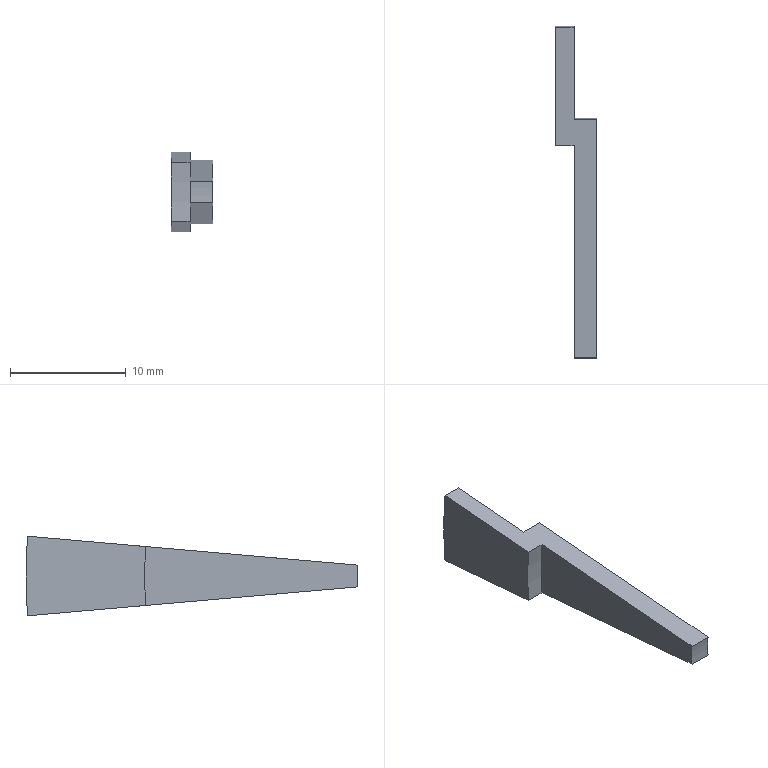Part | SolidWorks | features Revolution 1 | 1 solid | 10 faces | box 3.582 x 28.652 x 6.869 mm | volume 248.306 mm3 | plane 6 | cylinder 4 | commonest cylinder face diameters 21.59 x1 58.326 x1 62.852 x1 78.811 x1
STEP:
#1=CARTESIAN_POINT('',(-109.954,39.256,-3.434));
#2=VERTEX_POINT('',#1);
#3=CARTESIAN_POINT('',(-109.954,39.256,3.434));
#4=VERTEX_POINT('',#3);
#5=CARTESIAN_POINT('',(-109.954,0.,0.));
#6=DIRECTION('',(1.,0.,0.));
#7=DIRECTION('',(0.,0.,-1.));
#8=AXIS2_PLACEMENT_3D('',#5,#6,#7);
#9=CIRCLE('',#8,39.406);
#10=EDGE_CURVE('',#2,#4,#9,.T.);
#11=ORIENTED_EDGE('',*,*,#10,.F.);
#12=CARTESIAN_POINT('',(-111.582,39.256,-3.434));
#13=VERTEX_POINT('',#12);
#14=CARTESIAN_POINT('',(-111.582,39.256,-3.434));
#15=DIRECTION('',(-1.,0.,0.));
#16=VECTOR('',#15,1000.);
#17=LINE('',#14,#16);
#18=EDGE_CURVE('',#2,#13,#17,.T.);
#19=ORIENTED_EDGE('',*,*,#18,.T.);
#20=CARTESIAN_POINT('',(-111.582,39.256,3.434));
#21=VERTEX_POINT('',#20);
#22=CARTESIAN_POINT('',(-111.582,0.,0.));
#23=DIRECTION('',(1.,0.,0.));
#24=DIRECTION('',(0.,0.,-1.));
#25=AXIS2_PLACEMENT_3D('',#22,#23,#24);
#26=CIRCLE('',#25,39.406);
#27=EDGE_CURVE('',#13,#21,#26,.T.);
#28=ORIENTED_EDGE('',*,*,#27,.T.);
#29=CARTESIAN_POINT('',(-111.582,39.256,3.434));
#30=DIRECTION('',(-1.,0.,0.));
#31=VECTOR('',#30,1000.);
#32=LINE('',#29,#31);
#33=EDGE_CURVE('',#4,#21,#32,.T.);
#34=ORIENTED_EDGE('',*,*,#33,.F.);
#35=EDGE_LOOP('',(#11,#19,#28,#34));
#36=FACE_OUTER_BOUND('',#35,.T.);
#37=CARTESIAN_POINT('',(0.,0.,0.));
#38=DIRECTION('',(1.,0.,0.));
#39=DIRECTION('',(0.,0.,-1.));
#40=AXIS2_PLACEMENT_3D('',#37,#38,#39);
#41=CYLINDRICAL_SURFACE('',#40,39.406);
#42=ADVANCED_FACE('',(#36),#41,.T.);
#43=CARTESIAN_POINT('',(-109.954,31.306,-2.739));
#44=VERTEX_POINT('',#43);
#45=CARTESIAN_POINT('',(-109.954,31.306,2.739));
#46=VERTEX_POINT('',#45);
#47=CARTESIAN_POINT('',(-109.954,0.,0.));
#48=DIRECTION('',(1.,0.,0.));
#49=DIRECTION('',(0.,0.,-1.));
#50=AXIS2_PLACEMENT_3D('',#47,#48,#49);
#51=CIRCLE('',#50,31.426);
#52=EDGE_CURVE('',#44,#46,#51,.T.);
#53=ORIENTED_EDGE('',*,*,#52,.F.);
#54=CARTESIAN_POINT('',(-109.954,39.256,-3.434));
#55=DIRECTION('',(0.,0.9962,-0.08716));
#56=VECTOR('',#55,1000.);
#57=LINE('',#54,#56);
#58=EDGE_CURVE('',#44,#2,#57,.T.);
#59=ORIENTED_EDGE('',*,*,#58,.T.);
#60=ORIENTED_EDGE('',*,*,#10,.T.);
#61=CARTESIAN_POINT('',(-109.954,39.256,3.434));
#62=DIRECTION('',(0.,0.9962,0.08716));
#63=VECTOR('',#62,1000.);
#64=LINE('',#61,#63);
#65=EDGE_CURVE('',#46,#4,#64,.T.);
#66=ORIENTED_EDGE('',*,*,#65,.F.);
#67=EDGE_LOOP('',(#53,#59,#60,#66));
#68=FACE_OUTER_BOUND('',#67,.T.);
#69=CARTESIAN_POINT('',(-109.954,39.256,-3.434));
#70=DIRECTION('',(1.,0.,0.));
#71=DIRECTION('',(0.,0.,-1.));
#72=AXIS2_PLACEMENT_3D('',#69,#70,#71);
#73=PLANE('',#72);
#74=ADVANCED_FACE('',(#68),#73,.T.);
#75=CARTESIAN_POINT('',(-108.,31.306,-2.739));
#76=VERTEX_POINT('',#75);
#77=CARTESIAN_POINT('',(-108.,31.306,2.739));
#78=VERTEX_POINT('',#77);
#79=CARTESIAN_POINT('',(-108.,0.,0.));
#80=DIRECTION('',(1.,0.,0.));
#81=DIRECTION('',(0.,0.,-1.));
#82=AXIS2_PLACEMENT_3D('',#79,#80,#81);
#83=CIRCLE('',#82,31.426);
#84=EDGE_CURVE('',#76,#78,#83,.T.);
#85=ORIENTED_EDGE('',*,*,#84,.F.);
#86=CARTESIAN_POINT('',(-109.954,31.306,-2.739));
#87=DIRECTION('',(-1.,0.,0.));
#88=VECTOR('',#87,1000.);
#89=LINE('',#86,#88);
#90=EDGE_CURVE('',#76,#44,#89,.T.);
#91=ORIENTED_EDGE('',*,*,#90,.T.);
#92=ORIENTED_EDGE('',*,*,#52,.T.);
#93=CARTESIAN_POINT('',(-109.954,31.306,2.739));
#94=DIRECTION('',(-1.,0.,0.));
#95=VECTOR('',#94,1000.);
#96=LINE('',#93,#95);
#97=EDGE_CURVE('',#78,#46,#96,.T.);
#98=ORIENTED_EDGE('',*,*,#97,.F.);
#99=EDGE_LOOP('',(#85,#91,#92,#98));
#100=FACE_OUTER_BOUND('',#99,.T.);
#101=CARTESIAN_POINT('',(0.,0.,0.));
#102=DIRECTION('',(1.,0.,0.));
#103=DIRECTION('',(0.,0.,-1.));
#104=AXIS2_PLACEMENT_3D('',#101,#102,#103);
#105=CYLINDRICAL_SURFACE('',#104,31.426);
#106=ADVANCED_FACE('',(#100),#105,.T.);
#107=CARTESIAN_POINT('',(-108.,10.754,-0.9408));
#108=VERTEX_POINT('',#107);
#109=CARTESIAN_POINT('',(-108.,10.754,0.9408));
#110=VERTEX_POINT('',#109);
#111=CARTESIAN_POINT('',(-108.,0.,0.));
#112=DIRECTION('',(1.,0.,0.));
#113=DIRECTION('',(0.,0.,-1.));
#114=AXIS2_PLACEMENT_3D('',#111,#112,#113);
#115=CIRCLE('',#114,10.795);
#116=EDGE_CURVE('',#108,#110,#115,.T.);
#117=ORIENTED_EDGE('',*,*,#116,.F.);
#118=CARTESIAN_POINT('',(-108.,31.306,-2.739));
#119=DIRECTION('',(0.,0.9962,-0.08716));
#120=VECTOR('',#119,1000.);
#121=LINE('',#118,#120);
#122=EDGE_CURVE('',#108,#76,#121,.T.);
#123=ORIENTED_EDGE('',*,*,#122,.T.);
#124=ORIENTED_EDGE('',*,*,#84,.T.);
#125=CARTESIAN_POINT('',(-108.,31.306,2.739));
#126=DIRECTION('',(0.,0.9962,0.08716));
#127=VECTOR('',#126,1000.);
#128=LINE('',#125,#127);
#129=EDGE_CURVE('',#110,#78,#128,.T.);
#130=ORIENTED_EDGE('',*,*,#129,.F.);
#131=EDGE_LOOP('',(#117,#123,#124,#130));
#132=FACE_OUTER_BOUND('',#131,.T.);
#133=CARTESIAN_POINT('',(-108.,31.306,-2.739));
#134=DIRECTION('',(1.,0.,0.));
#135=DIRECTION('',(0.,0.,-1.));
#136=AXIS2_PLACEMENT_3D('',#133,#134,#135);
#137=PLANE('',#136);
#138=ADVANCED_FACE('',(#132),#137,.T.);
#139=CARTESIAN_POINT('',(-109.954,10.754,-0.9408));
#140=VERTEX_POINT('',#139);
#141=CARTESIAN_POINT('',(-109.954,10.754,0.9408));
#142=VERTEX_POINT('',#141);
#143=CARTESIAN_POINT('',(-109.954,0.,0.));
#144=DIRECTION('',(1.,0.,0.));
#145=DIRECTION('',(0.,0.,-1.));
#146=AXIS2_PLACEMENT_3D('',#143,#144,#145);
#147=CIRCLE('',#146,10.795);
#148=EDGE_CURVE('',#140,#142,#147,.T.);
#149=ORIENTED_EDGE('',*,*,#148,.F.);
#150=CARTESIAN_POINT('',(-108.,10.754,-0.9408));
#151=DIRECTION('',(1.,0.,0.));
#152=VECTOR('',#151,1000.);
#153=LINE('',#150,#152);
#154=EDGE_CURVE('',#140,#108,#153,.T.);
#155=ORIENTED_EDGE('',*,*,#154,.T.);
#156=ORIENTED_EDGE('',*,*,#116,.T.);
#157=CARTESIAN_POINT('',(-108.,10.754,0.9408));
#158=DIRECTION('',(1.,0.,0.));
#159=VECTOR('',#158,1000.);
#160=LINE('',#157,#159);
#161=EDGE_CURVE('',#142,#110,#160,.T.);
#162=ORIENTED_EDGE('',*,*,#161,.F.);
#163=EDGE_LOOP('',(#149,#155,#156,#162));
#164=FACE_OUTER_BOUND('',#163,.T.);
#165=CARTESIAN_POINT('',(0.,0.,0.));
#166=DIRECTION('',(1.,0.,0.));
#167=DIRECTION('',(0.,0.,-1.));
#168=AXIS2_PLACEMENT_3D('',#165,#166,#167);
#169=CYLINDRICAL_SURFACE('',#168,10.795);
#170=ADVANCED_FACE('',(#164),#169,.F.);
#171=CARTESIAN_POINT('',(-109.954,29.052,-2.542));
#172=VERTEX_POINT('',#171);
#173=CARTESIAN_POINT('',(-109.954,29.052,2.542));
#174=VERTEX_POINT('',#173);
#175=CARTESIAN_POINT('',(-109.954,0.,0.));
#176=DIRECTION('',(1.,0.,0.));
#177=DIRECTION('',(0.,0.,-1.));
#178=AXIS2_PLACEMENT_3D('',#175,#176,#177);
#179=CIRCLE('',#178,29.163);
#180=EDGE_CURVE('',#172,#174,#179,.T.);
#181=ORIENTED_EDGE('',*,*,#180,.F.);
#182=CARTESIAN_POINT('',(-109.954,29.052,-2.542));
#183=DIRECTION('',(0.,-0.9962,0.08716));
#184=VECTOR('',#183,1000.);
#185=LINE('',#182,#184);
#186=EDGE_CURVE('',#172,#140,#185,.T.);
#187=ORIENTED_EDGE('',*,*,#186,.T.);
#188=ORIENTED_EDGE('',*,*,#148,.T.);
#189=CARTESIAN_POINT('',(-109.954,29.052,2.542));
#190=DIRECTION('',(0.,-0.9962,-0.08716));
#191=VECTOR('',#190,1000.);
#192=LINE('',#189,#191);
#193=EDGE_CURVE('',#174,#142,#192,.T.);
#194=ORIENTED_EDGE('',*,*,#193,.F.);
#195=EDGE_LOOP('',(#181,#187,#188,#194));
#196=FACE_OUTER_BOUND('',#195,.T.);
#197=CARTESIAN_POINT('',(-109.954,29.052,-2.542));
#198=DIRECTION('',(-1.,0.,0.));
#199=DIRECTION('',(0.,0.,1.));
#200=AXIS2_PLACEMENT_3D('',#197,#198,#199);
#201=PLANE('',#200);
#202=ADVANCED_FACE('',(#196),#201,.T.);
#203=CARTESIAN_POINT('',(-111.582,29.052,-2.542));
#204=VERTEX_POINT('',#203);
#205=CARTESIAN_POINT('',(-111.582,29.052,2.542));
#206=VERTEX_POINT('',#205);
#207=CARTESIAN_POINT('',(-111.582,0.,0.));
#208=DIRECTION('',(1.,0.,0.));
#209=DIRECTION('',(0.,0.,-1.));
#210=AXIS2_PLACEMENT_3D('',#207,#208,#209);
#211=CIRCLE('',#210,29.163);
#212=EDGE_CURVE('',#204,#206,#211,.T.);
#213=ORIENTED_EDGE('',*,*,#212,.F.);
#214=CARTESIAN_POINT('',(-111.582,29.052,-2.542));
#215=DIRECTION('',(1.,0.,0.));
#216=VECTOR('',#215,1000.);
#217=LINE('',#214,#216);
#218=EDGE_CURVE('',#204,#172,#217,.T.);
#219=ORIENTED_EDGE('',*,*,#218,.T.);
#220=ORIENTED_EDGE('',*,*,#180,.T.);
#221=CARTESIAN_POINT('',(-111.582,29.052,2.542));
#222=DIRECTION('',(1.,0.,0.));
#223=VECTOR('',#222,1000.);
#224=LINE('',#221,#223);
#225=EDGE_CURVE('',#206,#174,#224,.T.);
#226=ORIENTED_EDGE('',*,*,#225,.F.);
#227=EDGE_LOOP('',(#213,#219,#220,#226));
#228=FACE_OUTER_BOUND('',#227,.T.);
#229=CARTESIAN_POINT('',(0.,0.,0.));
#230=DIRECTION('',(1.,0.,0.));
#231=DIRECTION('',(0.,0.,-1.));
#232=AXIS2_PLACEMENT_3D('',#229,#230,#231);
#233=CYLINDRICAL_SURFACE('',#232,29.163);
#234=ADVANCED_FACE('',(#228),#233,.F.);
#235=CARTESIAN_POINT('',(-111.582,29.052,-2.542));
#236=DIRECTION('',(0.,-0.9962,0.08716));
#237=VECTOR('',#236,1000.);
#238=LINE('',#235,#237);
#239=EDGE_CURVE('',#13,#204,#238,.T.);
#240=ORIENTED_EDGE('',*,*,#239,.T.);
#241=ORIENTED_EDGE('',*,*,#212,.T.);
#242=CARTESIAN_POINT('',(-111.582,29.052,2.542));
#243=DIRECTION('',(0.,-0.9962,-0.08716));
#244=VECTOR('',#243,1000.);
#245=LINE('',#242,#244);
#246=EDGE_CURVE('',#21,#206,#245,.T.);
#247=ORIENTED_EDGE('',*,*,#246,.F.);
#248=ORIENTED_EDGE('',*,*,#27,.F.);
#249=EDGE_LOOP('',(#240,#241,#247,#248));
#250=FACE_OUTER_BOUND('',#249,.T.);
#251=CARTESIAN_POINT('',(-111.582,29.052,-2.542));
#252=DIRECTION('',(-1.,0.,0.));
#253=DIRECTION('',(0.,0.,1.));
#254=AXIS2_PLACEMENT_3D('',#251,#252,#253);
#255=PLANE('',#254);
#256=ADVANCED_FACE('',(#250),#255,.T.);
#257=ORIENTED_EDGE('',*,*,#18,.F.);
#258=ORIENTED_EDGE('',*,*,#58,.F.);
#259=ORIENTED_EDGE('',*,*,#90,.F.);
#260=ORIENTED_EDGE('',*,*,#122,.F.);
#261=ORIENTED_EDGE('',*,*,#154,.F.);
#262=ORIENTED_EDGE('',*,*,#186,.F.);
#263=ORIENTED_EDGE('',*,*,#218,.F.);
#264=ORIENTED_EDGE('',*,*,#239,.F.);
#265=EDGE_LOOP('',(#257,#258,#259,#260,#261,#262,#263,#264));
#266=FACE_OUTER_BOUND('',#265,.T.);
#267=CARTESIAN_POINT('',(0.,0.,0.));
#268=DIRECTION('',(0.,-0.08716,-0.9962));
#269=DIRECTION('',(-1.,0.,0.));
#270=AXIS2_PLACEMENT_3D('',#267,#268,#269);
#271=PLANE('',#270);
#272=ADVANCED_FACE('',(#266),#271,.T.);
#273=ORIENTED_EDGE('',*,*,#33,.T.);
#274=ORIENTED_EDGE('',*,*,#246,.T.);
#275=ORIENTED_EDGE('',*,*,#225,.T.);
#276=ORIENTED_EDGE('',*,*,#193,.T.);
#277=ORIENTED_EDGE('',*,*,#161,.T.);
#278=ORIENTED_EDGE('',*,*,#129,.T.);
#279=ORIENTED_EDGE('',*,*,#97,.T.);
#280=ORIENTED_EDGE('',*,*,#65,.T.);
#281=EDGE_LOOP('',(#273,#274,#275,#276,#277,#278,#279,#280));
#282=FACE_OUTER_BOUND('',#281,.T.);
#283=CARTESIAN_POINT('',(0.,0.,0.));
#284=DIRECTION('',(0.,0.08716,-0.9962));
#285=DIRECTION('',(-1.,0.,0.));
#286=AXIS2_PLACEMENT_3D('',#283,#284,#285);
#287=PLANE('',#286);
#288=ADVANCED_FACE('',(#282),#287,.F.);
#289=CLOSED_SHELL('',(#42,#74,#106,#138,#170,#202,#234,#256,#272,#288));
#290=MANIFOLD_SOLID_BREP('',#289);
#291=CARTESIAN_POINT('',(0.,0.,0.));
#292=DIRECTION('',(0.,0.,1.));
#293=DIRECTION('',(1.,0.,0.));
#294=AXIS2_PLACEMENT_3D('',#291,#292,#293);
#295=(LENGTH_UNIT()NAMED_UNIT(*)SI_UNIT(.MILLI.,.METRE.));
#296=UNCERTAINTY_MEASURE_WITH_UNIT(LENGTH_MEASURE(0.00001),#295,'','');
#297=(NAMED_UNIT(*)PLANE_ANGLE_UNIT()SI_UNIT($,.RADIAN.));
#298=(NAMED_UNIT(*)SI_UNIT($,.STERADIAN.)SOLID_ANGLE_UNIT());
#299=(GEOMETRIC_REPRESENTATION_CONTEXT(3)GLOBAL_UNCERTAINTY_ASSIGNED_CONTEXT((#296))GLOBAL_UNIT_ASSIGNED_CONTEXT((#295,#297,#298))REPRESENTATION_CONTEXT('',''));
#300=ADVANCED_BREP_SHAPE_REPRESENTATION('',(#290,#294),#299);